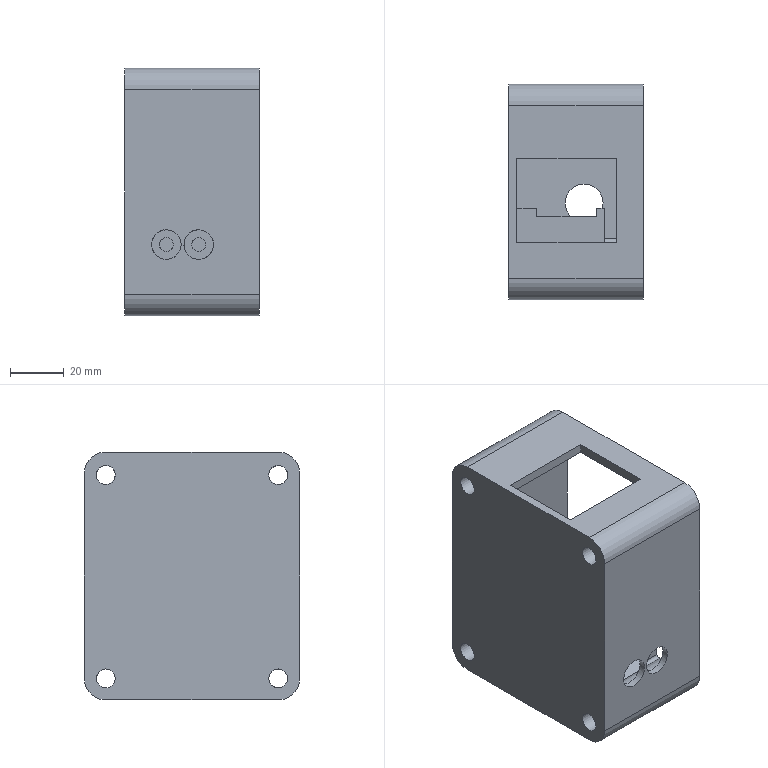CAM job | NX | 3+2 milling, drilling | part box 50 x 80 x 92 mm | stock box 66 x 100 x 97 mm
Tools:
number,name,description,diameter,corner_radius,flute_length,length,flutes
0,D1-10-D4-50-3T,D1*10*4*50-3T,1.0,0.0,10.0,11.0,3
9,D2-6-D4-50-3T-ROUGH,D2-6-D4-50-3T-粗,2.0,0.0,6.0,7.0,2
5,D4-12-D4-50-3T-ROUGH,D4-12-D4-50-3T-粗,4.0,0.0,12.0,50.0,2
7,D6-18-D6-50-3T-ROUGH,D6-18-D6-50-3T-粗,6.0,0.0,18.0,50.0,2
6,D12-36-D12-120-3T-FINISH,D12-55-D12-120-3T,12.0,0.0,45.0,120.0,3
1,D63面刀,D63面刀,63.0,0.0,30.0,30.0,4
2,点孔D8-120-90度,点孔D8-120-90度,8.0,0.0,0.0,120.0,2
13,钻头D2.5-35-61,钻刀D2.5-35-61,2.5,0.0,36.0,61.0,2
4,钻头D4.0-54-83,钻刀D4.0-54-83,4.0,0.0,54.0,83.0,2
0,钻头D5.1-62-92,钻刀D5.1-62-92,5.1,0.0,62.0,92.0,2
3,钻头D7.0-73-105,钻刀D7.0-73-105,7.0,0.0,73.0,105.0,2
14,上排M3-10-D4-52,上排M3-10-D4-52,3.0,0.0,10.0,12.0,2
12,倒角D5-90度,倒角D5-90度,5.0,0.0,5.0,50.0,2
10,D10-1,Milling Tool-T Cutter,16.0,,4.0,50.0,4
Operations:
program,operation,operation_type,tool,method,geometry_group,spindle_rpm,surface_speed,feed_per_tooth,feed_cut,feed_plunge,cut_length_mm,path_length_mm,cut_time_min,machine_time_min
A1,PLANAR_MILL_1,PlanarMilling,D63面刀,METHOD,WORKPIECE_54,4000.0,791.0,0.0625,1000.0,100.0,464.0,804.596,0.464,0.4981
A1,DRILLING_COPY,Operation,点孔D8-120-90度,METHOD,WORKPIECE_54,3000.0,75.0,0.0333,200.0,0.0,81.0,534.312,0.405,0.4503
A1,DRILLING_COPY_COPY_1,Operation,点孔D8-120-90度,METHOD,WORKPIECE_54,3000.0,75.0,0.0333,200.0,0.0,18.0,308.7,0.09,0.1191
A1,DRILLING_COPY_COPY_1_COPY,Operation,钻头D7.0-73-105,METHOD,WORKPIECE_54,3000.0,65.0,0.0417,250.0,0.0,228.0,728.7,0.912,0.9621
A1,DRILLING_COPY_COPY,Operation,钻头D4.0-54-83,METHOD,WORKPIECE_54,3000.0,37.0,0.0333,200.0,0.0,900.0,2172.312,4.5,4.627
A1,DRILLING_COPY_COPY_COPY,Operation,D4-12-D4-50-3T-ROUGH,METHOD,WORKPIECE_54,2000.0,25.0,0.0375,150.0,0.0,900.0,2172.312,6.0,6.127
A1,ADAPTIVE_MILLING,CavityMilling,D12-36-D12-120-3T-FINISH,METHOD,WORKPIECE_54,6500.0,245.0,0.1026,2000.0,100.0,34492.841,35831.275,16.929,17.062
A1,PLANAR_MILL_5,PlanarMilling,D12-36-D12-120-3T-FINISH,METHOD,WORKPIECE_54,3000.0,113.0,0.0889,800.0,100.0,1512.991,1780.491,1.891,1.918
A1,ADAPTIVE_MILLING_COPY,CavityMilling,D6-18-D6-50-3T-ROUGH,METHOD,WORKPIECE_54,4500.0,84.0,0.1667,1500.0,100.0,39574.395,45795.516,26.272,26.894
A1,PLANAR_MILL_COPY_1_COPY,PlanarMilling,D6-18-D6-50-3T-ROUGH,METHOD,WORKPIECE_54,4000.0,75.0,0.1,800.0,100.0,733.937,885.937,0.9174,0.9326
A1,PLANAR_MILL_2_COPY,PlanarMilling,D6-18-D6-50-3T-ROUGH,METHOD,WORKPIECE_54,4000.0,75.0,0.1,800.0,100.0,1119.118,1825.984,1.399,1.47
A1,PLANAR_MILL_COPY_COPY_2,PlanarMilling,D6-18-D6-50-3T-ROUGH,METHOD,WORKPIECE_54,4000.0,75.0,0.1,800.0,100.0,296.859,367.859,0.3711,0.3782
A1,PLANAR_MILL_COPY_COPY,PlanarMilling,D6-18-D6-50-3T-ROUGH,METHOD,WORKPIECE_54,4000.0,75.0,0.1,800.0,100.0,326.625,767.371,0.4083,0.4524
A1,PLANAR_MILL_2_COPY_2,PlanarMilling,D6-18-D6-50-3T-ROUGH,METHOD,WORKPIECE_54,4000.0,75.0,0.1,800.0,100.0,520.798,767.798,0.651,0.6757
A1,FLOOR_FACING,VolumeBased25DMillingOperation,D6-18-D6-50-3T-ROUGH,METHOD,WORKPIECE_54,4000.0,75.0,0.1,800.0,100.0,130.697,213.697,0.1634,0.1717
A1,PLANAR_MILL_COPY_1,PlanarMilling,D6-18-D6-50-3T-ROUGH,METHOD,WORKPIECE_54,4000.0,75.0,0.1,800.0,100.0,1332.358,1482.358,1.665,1.68
A1,PLANAR_MILL_2,PlanarMilling,D6-18-D6-50-3T-ROUGH,METHOD,WORKPIECE_54,4000.0,75.0,0.1,800.0,100.0,1554.393,1921.393,1.943,1.98
A1,PLANAR_MILL_2_COPY_1,PlanarMilling,D4-12-D4-50-3T-ROUGH,METHOD,WORKPIECE_54,2500.0,31.0,0.06,300.0,100.0,2111.326,3597.601,7.038,7.186
A1,PLANAR_MILL_COPY_2,PlanarMilling,D4-12-D4-50-3T-ROUGH,METHOD,WORKPIECE_54,2500.0,31.0,0.06,300.0,100.0,2483.783,4645.822,8.279,8.495
A1,PLANAR_MILL_COPY_COPY_1,PlanarMilling,D2-6-D4-50-3T-ROUGH,METHOD,WORKPIECE_54,6500.0,40.0,0.0231,300.0,100.0,1505.063,2290.052,5.017,5.095
A1,PLANAR_MILL_COPY_COPY_1_COPY,PlanarMilling,D2-6-D4-50-3T-ROUGH,METHOD,WORKPIECE_54,6500.0,40.0,0.0231,300.0,100.0,163.919,316.832,0.5464,0.5617
A1,PLANAR_MILL_4,PlanarMilling,D10-1,METHOD,WORKPIECE_54,1600.0,80.0,0.0938,600.0,100.0,266.549,995.349,0.4442,0.5171
A1,PLANAR_PROFILING,PlanarMilling,D10-1,METHOD,WORKPIECE_54,1600.0,80.0,0.125,800.0,100.0,727.38,2951.78,0.9092,1.132
A1,PLANAR_PROFILING_COPY,PlanarMilling,D10-1,METHOD,WORKPIECE_54,3000.0,94.0,0.0667,800.0,100.0,306.265,1243.416,0.3828,0.4765
A1,PLANAR_PROFILING_COPY_COPY_COPY,PlanarMilling,D10-1,METHOD,WORKPIECE_54,3000.0,94.0,0.0667,800.0,100.0,38.283,137.583,0.0479,0.0578
A1,PLANAR_PROFILING_COPY_COPY,PlanarMilling,D10-1,METHOD,WORKPIECE_54,3000.0,94.0,0.0667,800.0,100.0,38.283,172.983,0.0479,0.0613
A1,DRILLING,Operation,倒角D5-90度,METHOD,WORKPIECE_54,3000.0,47.0,0.0333,200.0,0.0,27.0,356.531,0.135,0.168
A1,PLANAR_MILL_3,PlanarMilling,倒角D5-90度,METHOD,WORKPIECE_54,3000.0,47.0,0.1667,1000.0,100.0,349.973,408.973,0.35,0.3559
A1,PLANAR_MILL_3_COPY_1,PlanarMilling,倒角D5-90度,METHOD,WORKPIECE_54,3000.0,47.0,0.1667,1000.0,100.0,77.927,525.454,0.0779,0.1227
A1,PLANAR_MILL_3_COPY,PlanarMilling,倒角D5-90度,METHOD,WORKPIECE_54,3000.0,47.0,0.1667,1000.0,100.0,312.281,371.281,0.3123,0.3182
A1,PLANAR_MILL_3_COPY_COPY,PlanarMilling,倒角D5-90度,METHOD,WORKPIECE_54,3000.0,47.0,0.1667,1000.0,100.0,247.994,322.994,0.248,0.2555
A1,PLANAR_MILL_3_COPY_COPY_COPY,PlanarMilling,倒角D5-90度,METHOD,WORKPIECE_54,3000.0,47.0,0.1667,1000.0,100.0,115.029,321.037,0.115,0.1356
A1,DRILLING_COPY_1,Operation,钻头D2.5-35-61,METHOD,WORKPIECE_54,3000.0,23.0,0.025,150.0,0.0,60.0,422.531,0.4,0.4363
A1,DRILLING_COPY_1_COPY,Operation,上排M3-10-D4-52,METHOD,WORKPIECE_54,300.0,2.0,0.0008,0.5,0.0,54.0,410.531,108.0,108.036
B1,PLANAR_MILL,PlanarMilling,D63面刀,METHOD,B-G55,3500.0,692.0,0.0714,1000.0,100.0,4992.0,10334.045,4.992,5.526
B1,PLANAR_MILL_COPY,PlanarMilling,D63面刀,METHOD,B-G55,3500.0,692.0,0.0429,600.0,100.0,416.0,689.506,0.6933,0.7207
B1,PLANAR_MILL_6,PlanarMilling,倒角D5-90度,METHOD,B-G55,3500.0,54.0,0.1429,1000.0,100.0,353.115,393.115,0.3531,0.3571
B1,PLANAR_MILL_6_COPY,PlanarMilling,倒角D5-90度,METHOD,B-G55,3500.0,54.0,0.1143,800.0,100.0,86.83,446.356,0.1085,0.1445
C1,HOLE_MILLING,CylinderMilling,D6-18-D6-50-3T-ROUGH,METHOD,C-G56,4000.0,75.0,0.1,800.0,100.0,585.01,682.01,0.7313,0.741
C1,HOLE_MILLING_COPY,CylinderMilling,D6-18-D6-50-3T-ROUGH,METHOD,C-G56,4000.0,75.0,0.1,800.0,100.0,47.124,151.124,0.0589,0.0693
C1,DRILLING_1,Operation,点孔D8-120-90度,METHOD,C-G56,2000.0,50.0,0.05,200.0,0.0,11.8,108.969,0.059,0.0687
C1,DRILLING_1_COPY,Operation,钻头D5.1-62-92,METHOD,C-G56,2000.0,50.0,0.05,200.0,0.0,46.0,177.369,0.23,0.2431
D1,PLANAR_MILL_7,PlanarMilling,D6-18-D6-50-3T-ROUGH,METHOD,D-G57,4500.0,84.0,0.1667,1500.0,100.0,2596.02,2659.52,1.731,1.737
D1,PLANAR_MILL_7_COPY,PlanarMilling,D6-18-D6-50-3T-ROUGH,METHOD,D-G57,4500.0,84.0,0.0667,600.0,100.0,123.283,196.283,0.2055,0.2128
D1,PLANAR_MILL_7_COPY_COPY,PlanarMilling,D2-6-D4-50-3T-ROUGH,METHOD,D-G57,4500.0,84.0,0.0667,600.0,100.0,761.027,1289.787,1.268,1.321
E1,PLANAR_MILL_8,PlanarMilling,D6-18-D6-50-3T-ROUGH,METHOD,E-G58,4500.0,84.0,0.0889,800.0,100.0,398.574,462.074,0.4982,0.5046
E1,PLANAR_MILL_8_COPY_1,PlanarMilling,D6-18-D6-50-3T-ROUGH,METHOD,E-G58,4500.0,84.0,0.0889,800.0,100.0,223.5,283.7,0.2794,0.2854
E1,PLANAR_MILL_8_COPY,PlanarMilling,D6-18-D6-50-3T-ROUGH,METHOD,E-G58,4500.0,84.0,0.0667,600.0,100.0,32.926,99.926,0.0549,0.0616
E1,PLANAR_MILL_8_COPY_1_COPY,PlanarMilling,D2-6-D4-50-3T-ROUGH,METHOD,E-G58,4500.0,84.0,0.0889,800.0,100.0,421.045,481.245,0.5263,0.5323
E1,PLANAR_MILL_8_COPY_1_COPY_COPY,PlanarMilling,D1-10-D4-50-3T,METHOD,E-G58,4500.0,84.0,0.0889,800.0,100.0,668.623,728.823,0.8358,0.8418